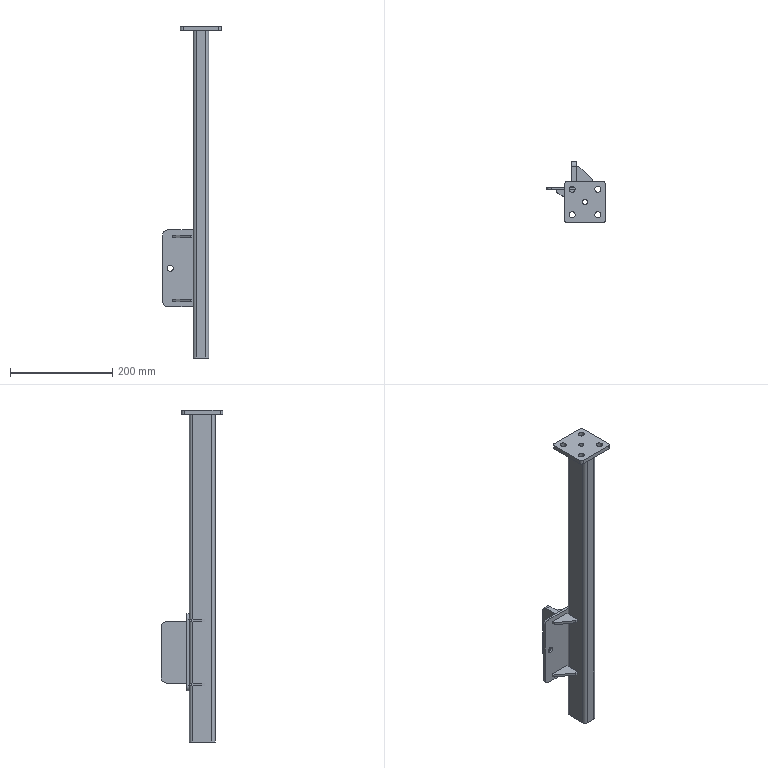Part | SolidWorks | features Gusset 4, Cut 1, Extrusion 1, Fillet 1, FlatPattern 1, ICE 1, SMBaseFlange 1, SheetMetal 1, WeldMemberFeat 1, WeldmentFeature 1 | 8 solids | 84 faces | box 115 x 120 x 648 mm | volume 459448 mm3 | plane 56 | cylinder 28 | commonest cylinder face diameters 12 x14 10 x6 6 x4 20 x4